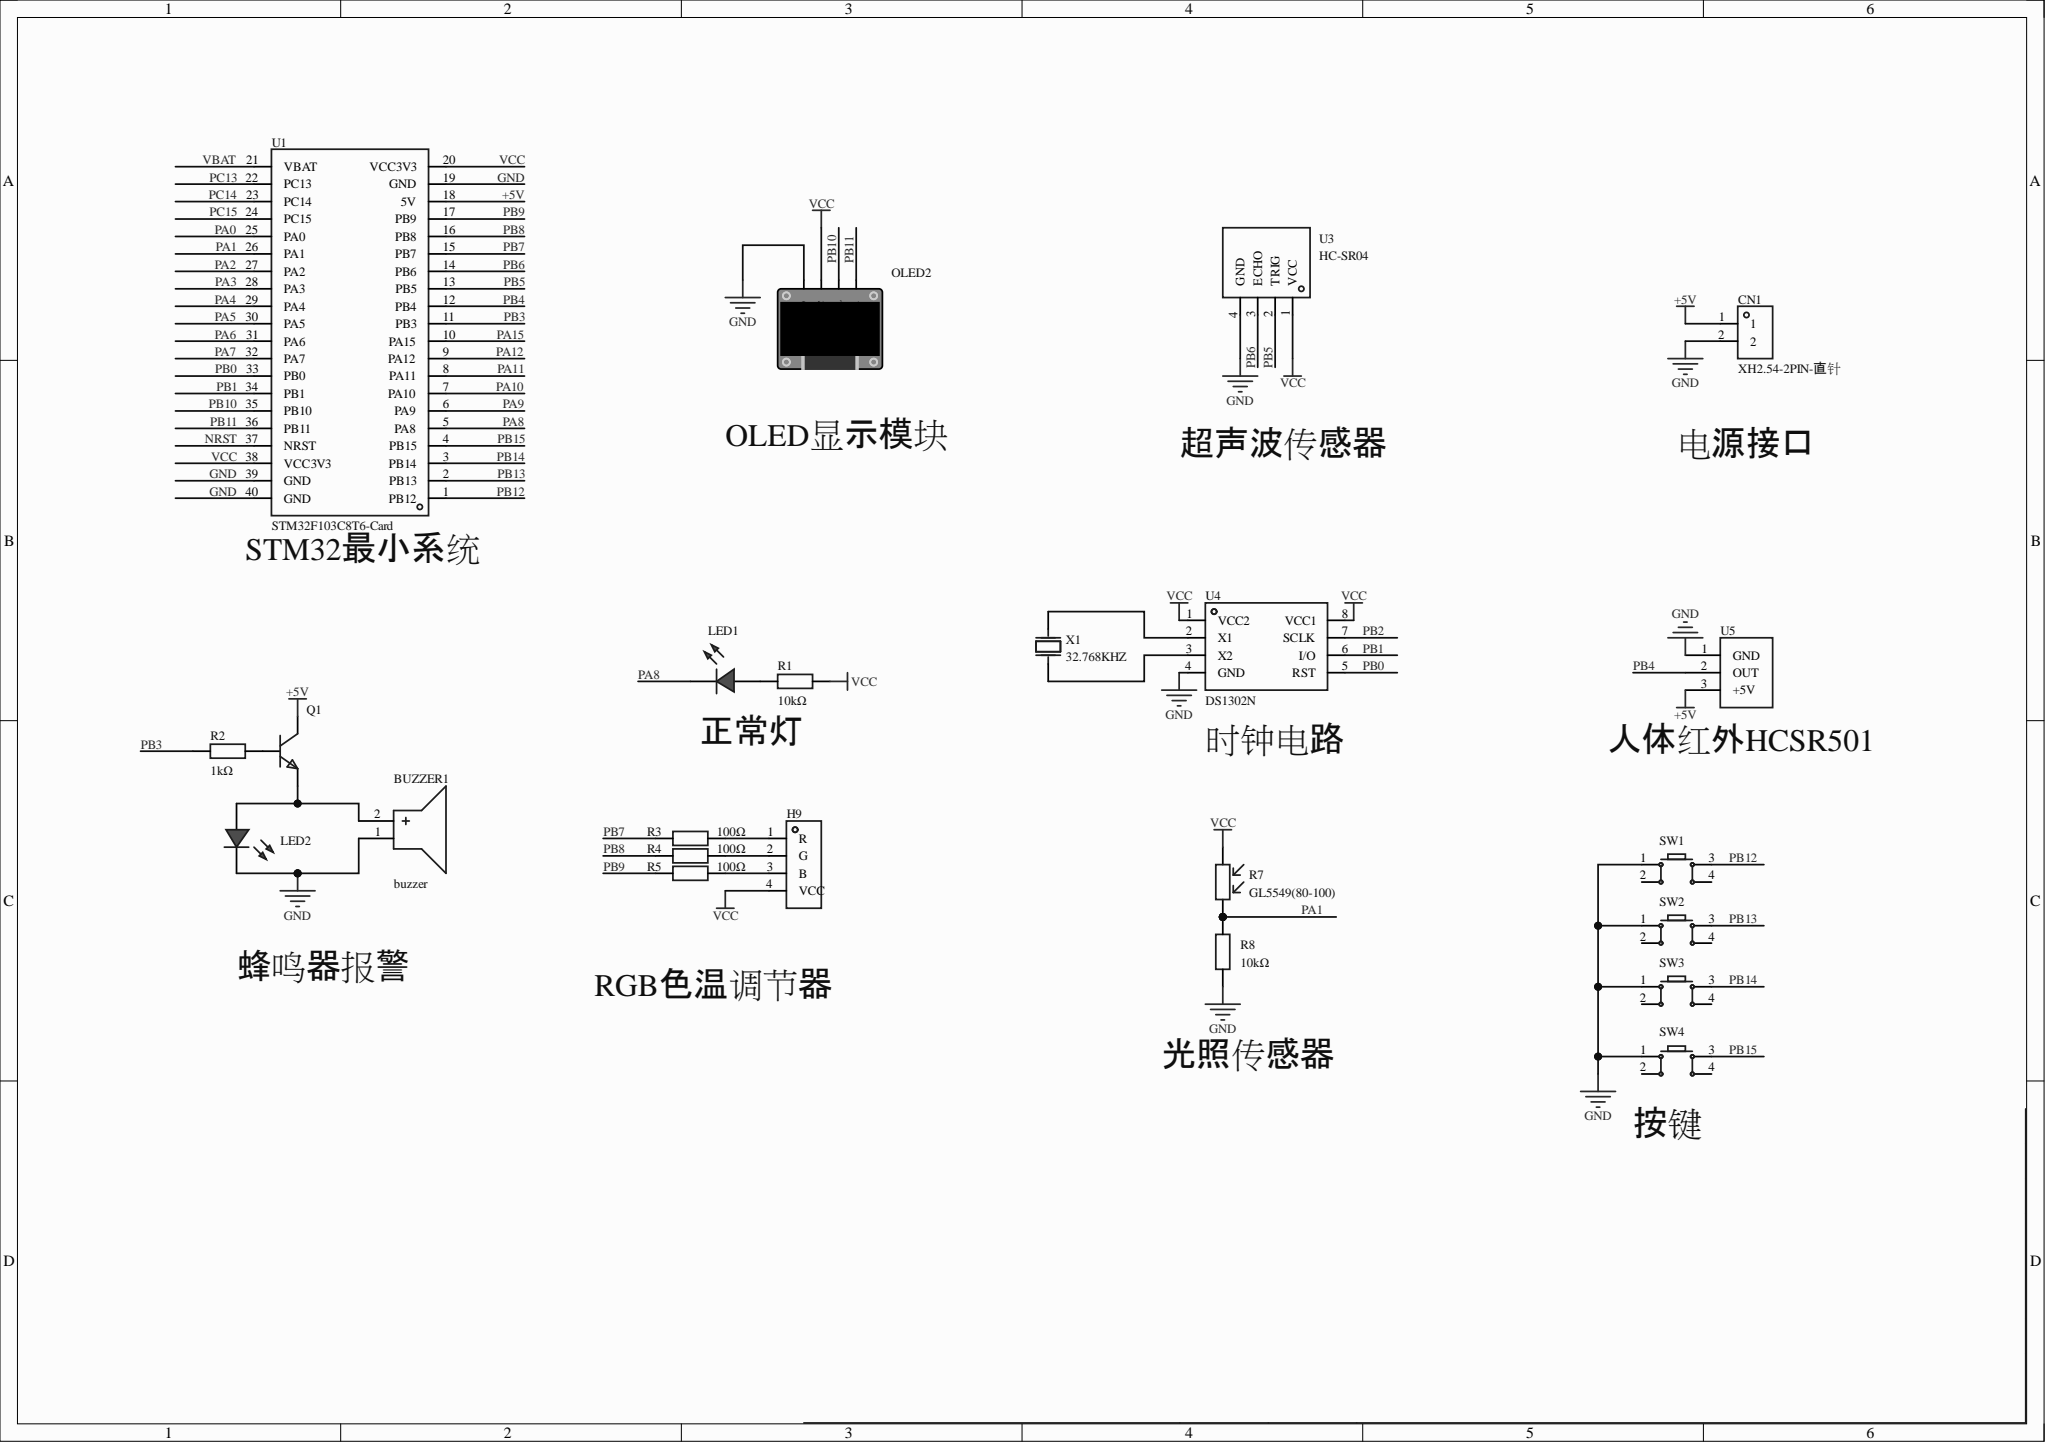Circuit board | Altium Designer | 23 parts | 28 nets
Bill of materials:
Comment,Description,Designator,Footprint,LibRef,Quantity
"buzzer","","BUZZER1","BUZ-TH_BD12.0-P6.00-D0.9-RD","buzzer","1"
"XH2.54-2PIN-直针","","CN1","CONN-TH_XH2.54-2P","XH2.54-2PIN-直针","1"
"","","H9","HDR-TH_4P-P2.54-V-F","HDR-F_2.54_1x4P","1"
"","","LED1, LED2","LED_TH-3mm","LED_TH-R_3mm","2"
"","","OLED2","0.96OLED_4P","0.96OLED模块_4P","1"
"","","Q1","S8050_TO_92","S8050_TO_NPN","1"
"10kΩ","","R1, R8","Res_1/8W","Res_AXIAL-1/8W","2"
"1kΩ","","R2","Res_1/8W","Res_AXIAL-1/8W","1"
"100Ω","","R3, R4, R5","Res_1/8W","Res_AXIAL-1/8W","3"
"GL5549(80-100)","","R7","RES-TH_L5.1-W4.3-P3.40-D0.5","GL5549(80-100)","1"
"","","SW1, SW2, SW3, SW4","SW-TH_4P-L6.0-W6.0-P4.50-LS6.5","Key_TH_6x6x6","4"
"STM32F103C8T6-Card","","U1","CONN-TH_L53.3-W22.9_STM32F103C8T6-CARD","STM32F103C8T6-Card","1"
"HC-SR04","","U3","TH_HC-SR04V","HC-SR04","1"
"DS1302N","","U4","DIP-8_L9.7-W6.4-P2.54-LS7.6-BL","DS1302N","1"
"","","U5","HC-SR501","HCSR501","1"
"32.768KHZ","","X1","HC-49S_L11.5-W5.0-P4.88","8MHZ","1"
Netlist (Protel format):
[
BUZZER1
BUZ-TH_BD12.0-P6.00-D0.9-RD
buzzer



]
[
CN1
CONN-TH_XH2.54-2P
XH2.54-2PIN-直针



]
[
H9
HDR-TH_4P-P2.54-V-F




]
[
LED1
LED_TH-3mm




]
[
LED2
LED_TH-3mm




]
[
OLED2
0.96OLED_4P




]
[
Q1
S8050_TO_92




]
[
R1
Res_1/8W
10kΩ



]
[
R2
Res_1/8W
1kΩ



]
[
R3
Res_1/8W
100Ω



]
[
R4
Res_1/8W
100Ω



]
[
R5
Res_1/8W
100Ω



]
[
R7
RES-TH_L5.1-W4.3-P3.40-D0.5
GL5549(80-100)



]
[
R8
Res_1/8W
10kΩ



]
[
SW1
SW-TH_4P-L6.0-W6.0-P4.50-LS6.5




]
[
SW2
SW-TH_4P-L6.0-W6.0-P4.50-LS6.5




]
[
SW3
SW-TH_4P-L6.0-W6.0-P4.50-LS6.5




]
[
SW4
SW-TH_4P-L6.0-W6.0-P4.50-LS6.5




]
[
U1
CONN-TH_L53.3-W22.9_STM32F103C8T6-CARD
STM32F103C8T6-Card



]
[
U3
TH_HC-SR04V
HC-SR04



]
[
U4
DIP-8_L9.7-W6.4-P2.54-LS7.6-BL
DS1302N



]
[
U5
HC-SR501




]
[
X1
HC-49S_L11.5-W5.0-P4.88
32.768KHZ



]
(
VCC
H9-4
OLED2-2
R1-2
R7-1
U1-20
U1-38
U3-1
U4-1
U4-8
)
(
PB15
SW4-3
U1-4
)
(
PB14
SW3-3
U1-3
)
(
PB13
SW2-3
U1-2
)
(
PB12
SW1-3
U1-1
)
(
PB11
OLED2-4
U1-36
)
(
PB10
OLED2-3
U1-35
)
(
PB9
R5-1
U1-17
)
(
PB8
R4-1
U1-16
)
(
PB7
R3-1
U1-15
)
(
PB6
U1-14
U3-3
)
(
PB5
U1-13
U3-2
)
(
PB4
U1-12
U5-2
)
(
PB3
R2-1
U1-11
)
(
PB1
U1-34
U4-6
)
(
PB0
U1-33
U4-5
)
(
PA8
LED1-2
U1-5
)
(
PA1
R7-2
R8-2
U1-26
)
(
NetU4_3
U4-3
X1-1
)
(
NetU4_2
U4-2
X1-2
)
(
NetQ1_2
Q1-2
R2-2
)
(
NetLED1_1
LED1-1
R1-1
)
(
NetH9_3
H9-3
R5-2
)
(
NetH9_2
H9-2
R4-2
)
(
NetH9_1
H9-1
R3-2
)
(
NetBUZZER1_2
BUZZER1-2
LED2-1
Q1-1
)
(
GND
BUZZER1-1
CN1-2
LED2-2
OLED2-1
R8-1
SW1-1
SW2-1
SW3-1
SW4-1
U1-19
U1-39
U1-40
U3-4
U4-4
U5-1
)
(
+5V
CN1-1
Q1-3
U1-18
U5-3
)